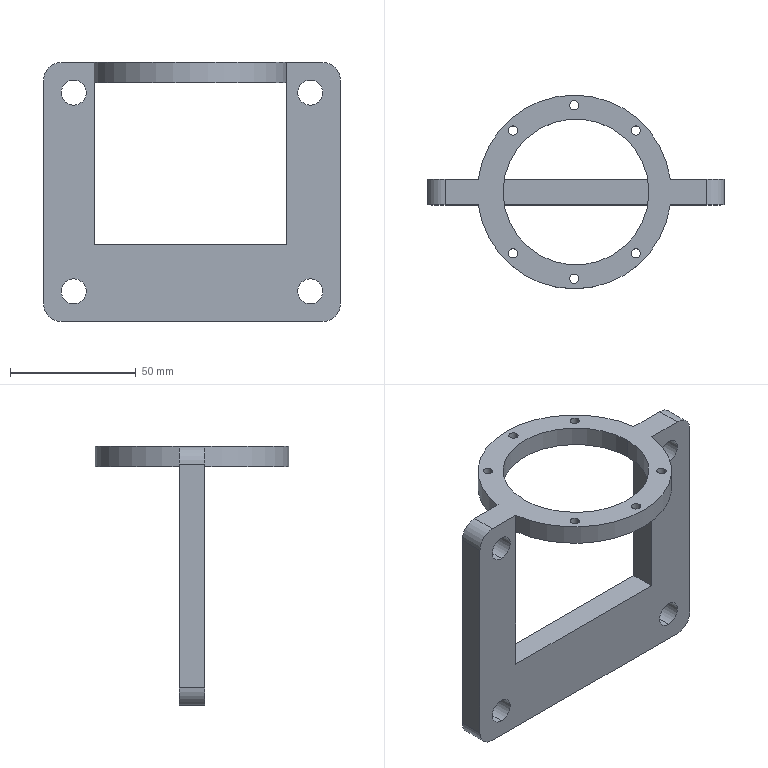Part | SolidWorks | features ICE 4, Extrusion 1, Fillet 1 | 1 solid | 38 faces | box 118 x 77 x 103 mm | volume 78200 mm3 | cylinder 28 | plane 10 | commonest cylinder face diameters 3.7 x12 10 x8 14 x4 58 x2 77 x2
STEP:
#1=CARTESIAN_POINT('',(-46.321,-5.,-9.));
#2=VERTEX_POINT('',#1);
#3=CARTESIAN_POINT('',(-46.321,-5.,1.));
#4=VERTEX_POINT('',#3);
#5=CARTESIAN_POINT('',(-46.321,-5.,-4.));
#6=DIRECTION('',(0.,1.,0.));
#7=DIRECTION('',(0.,0.,-1.));
#8=AXIS2_PLACEMENT_3D('',#5,#6,#7);
#9=CIRCLE('',#8,5.);
#10=EDGE_CURVE('',#2,#4,#9,.T.);
#11=ORIENTED_EDGE('',*,*,#10,.F.);
#12=CARTESIAN_POINT('',(-46.321,5.,-9.));
#13=VERTEX_POINT('',#12);
#14=CARTESIAN_POINT('',(-46.321,-38.501,-9.));
#15=DIRECTION('',(0.,1.,0.));
#16=VECTOR('',#15,1000.);
#17=LINE('',#14,#16);
#18=EDGE_CURVE('',#2,#13,#17,.T.);
#19=ORIENTED_EDGE('',*,*,#18,.T.);
#20=CARTESIAN_POINT('',(-46.321,5.,1.));
#21=VERTEX_POINT('',#20);
#22=CARTESIAN_POINT('',(-46.321,5.,-4.));
#23=DIRECTION('',(0.,1.,0.));
#24=DIRECTION('',(0.,0.,1.));
#25=AXIS2_PLACEMENT_3D('',#22,#23,#24);
#26=CIRCLE('',#25,5.);
#27=EDGE_CURVE('',#13,#21,#26,.T.);
#28=ORIENTED_EDGE('',*,*,#27,.T.);
#29=CARTESIAN_POINT('',(-46.321,-38.501,1.));
#30=DIRECTION('',(0.,1.,0.));
#31=VECTOR('',#30,1000.);
#32=LINE('',#29,#31);
#33=EDGE_CURVE('',#4,#21,#32,.T.);
#34=ORIENTED_EDGE('',*,*,#33,.F.);
#35=EDGE_LOOP('',(#11,#19,#28,#34));
#36=FACE_OUTER_BOUND('',#35,.T.);
#37=CARTESIAN_POINT('',(-46.321,-38.501,-4.));
#38=DIRECTION('',(0.,1.,0.));
#39=DIRECTION('',(0.,0.,1.));
#40=AXIS2_PLACEMENT_3D('',#37,#38,#39);
#41=CYLINDRICAL_SURFACE('',#40,5.);
#42=ADVANCED_FACE('',(#36),#41,.F.);
#43=CARTESIAN_POINT('',(47.679,-5.,-88.));
#44=VERTEX_POINT('',#43);
#45=CARTESIAN_POINT('',(47.679,-5.,-78.));
#46=VERTEX_POINT('',#45);
#47=CARTESIAN_POINT('',(47.679,-5.,-83.));
#48=DIRECTION('',(0.,1.,0.));
#49=DIRECTION('',(0.,0.,-1.));
#50=AXIS2_PLACEMENT_3D('',#47,#48,#49);
#51=CIRCLE('',#50,5.);
#52=EDGE_CURVE('',#44,#46,#51,.T.);
#53=ORIENTED_EDGE('',*,*,#52,.F.);
#54=CARTESIAN_POINT('',(47.679,5.,-88.));
#55=VERTEX_POINT('',#54);
#56=CARTESIAN_POINT('',(47.679,-38.501,-88.));
#57=DIRECTION('',(0.,1.,0.));
#58=VECTOR('',#57,1000.);
#59=LINE('',#56,#58);
#60=EDGE_CURVE('',#44,#55,#59,.T.);
#61=ORIENTED_EDGE('',*,*,#60,.T.);
#62=CARTESIAN_POINT('',(47.679,5.,-78.));
#63=VERTEX_POINT('',#62);
#64=CARTESIAN_POINT('',(47.679,5.,-83.));
#65=DIRECTION('',(0.,1.,0.));
#66=DIRECTION('',(0.,0.,1.));
#67=AXIS2_PLACEMENT_3D('',#64,#65,#66);
#68=CIRCLE('',#67,5.);
#69=EDGE_CURVE('',#55,#63,#68,.T.);
#70=ORIENTED_EDGE('',*,*,#69,.T.);
#71=CARTESIAN_POINT('',(47.679,-38.501,-78.));
#72=DIRECTION('',(0.,1.,0.));
#73=VECTOR('',#72,1000.);
#74=LINE('',#71,#73);
#75=EDGE_CURVE('',#46,#63,#74,.T.);
#76=ORIENTED_EDGE('',*,*,#75,.F.);
#77=EDGE_LOOP('',(#53,#61,#70,#76));
#78=FACE_OUTER_BOUND('',#77,.T.);
#79=CARTESIAN_POINT('',(47.679,-38.501,-83.));
#80=DIRECTION('',(0.,1.,0.));
#81=DIRECTION('',(0.,0.,1.));
#82=AXIS2_PLACEMENT_3D('',#79,#80,#81);
#83=CYLINDRICAL_SURFACE('',#82,5.);
#84=ADVANCED_FACE('',(#78),#83,.F.);
#85=CARTESIAN_POINT('',(47.679,-5.,-9.));
#86=VERTEX_POINT('',#85);
#87=CARTESIAN_POINT('',(47.679,-5.,1.));
#88=VERTEX_POINT('',#87);
#89=CARTESIAN_POINT('',(47.679,-5.,-4.));
#90=DIRECTION('',(0.,1.,0.));
#91=DIRECTION('',(0.,0.,-1.));
#92=AXIS2_PLACEMENT_3D('',#89,#90,#91);
#93=CIRCLE('',#92,5.);
#94=EDGE_CURVE('',#86,#88,#93,.T.);
#95=ORIENTED_EDGE('',*,*,#94,.F.);
#96=CARTESIAN_POINT('',(47.679,5.,-9.));
#97=VERTEX_POINT('',#96);
#98=CARTESIAN_POINT('',(47.679,-38.501,-9.));
#99=DIRECTION('',(0.,1.,0.));
#100=VECTOR('',#99,1000.);
#101=LINE('',#98,#100);
#102=EDGE_CURVE('',#86,#97,#101,.T.);
#103=ORIENTED_EDGE('',*,*,#102,.T.);
#104=CARTESIAN_POINT('',(47.679,5.,1.));
#105=VERTEX_POINT('',#104);
#106=CARTESIAN_POINT('',(47.679,5.,-4.));
#107=DIRECTION('',(0.,1.,0.));
#108=DIRECTION('',(0.,0.,1.));
#109=AXIS2_PLACEMENT_3D('',#106,#107,#108);
#110=CIRCLE('',#109,5.);
#111=EDGE_CURVE('',#97,#105,#110,.T.);
#112=ORIENTED_EDGE('',*,*,#111,.T.);
#113=CARTESIAN_POINT('',(47.679,-38.501,1.));
#114=DIRECTION('',(0.,1.,0.));
#115=VECTOR('',#114,1000.);
#116=LINE('',#113,#115);
#117=EDGE_CURVE('',#88,#105,#116,.T.);
#118=ORIENTED_EDGE('',*,*,#117,.F.);
#119=EDGE_LOOP('',(#95,#103,#112,#118));
#120=FACE_OUTER_BOUND('',#119,.T.);
#121=CARTESIAN_POINT('',(47.679,-38.501,-4.));
#122=DIRECTION('',(0.,1.,0.));
#123=DIRECTION('',(0.,0.,1.));
#124=AXIS2_PLACEMENT_3D('',#121,#122,#123);
#125=CYLINDRICAL_SURFACE('',#124,5.);
#126=ADVANCED_FACE('',(#120),#125,.F.);
#127=CARTESIAN_POINT('',(-46.321,-5.,-88.));
#128=VERTEX_POINT('',#127);
#129=CARTESIAN_POINT('',(-46.321,-5.,-78.));
#130=VERTEX_POINT('',#129);
#131=CARTESIAN_POINT('',(-46.321,-5.,-83.));
#132=DIRECTION('',(0.,1.,0.));
#133=DIRECTION('',(0.,0.,-1.));
#134=AXIS2_PLACEMENT_3D('',#131,#132,#133);
#135=CIRCLE('',#134,5.);
#136=EDGE_CURVE('',#128,#130,#135,.T.);
#137=ORIENTED_EDGE('',*,*,#136,.F.);
#138=CARTESIAN_POINT('',(-46.321,5.,-88.));
#139=VERTEX_POINT('',#138);
#140=CARTESIAN_POINT('',(-46.321,-38.501,-88.));
#141=DIRECTION('',(0.,1.,0.));
#142=VECTOR('',#141,1000.);
#143=LINE('',#140,#142);
#144=EDGE_CURVE('',#128,#139,#143,.T.);
#145=ORIENTED_EDGE('',*,*,#144,.T.);
#146=CARTESIAN_POINT('',(-46.321,5.,-78.));
#147=VERTEX_POINT('',#146);
#148=CARTESIAN_POINT('',(-46.321,5.,-83.));
#149=DIRECTION('',(0.,1.,0.));
#150=DIRECTION('',(0.,0.,1.));
#151=AXIS2_PLACEMENT_3D('',#148,#149,#150);
#152=CIRCLE('',#151,5.);
#153=EDGE_CURVE('',#139,#147,#152,.T.);
#154=ORIENTED_EDGE('',*,*,#153,.T.);
#155=CARTESIAN_POINT('',(-46.321,-38.501,-78.));
#156=DIRECTION('',(0.,1.,0.));
#157=VECTOR('',#156,1000.);
#158=LINE('',#155,#157);
#159=EDGE_CURVE('',#130,#147,#158,.T.);
#160=ORIENTED_EDGE('',*,*,#159,.F.);
#161=EDGE_LOOP('',(#137,#145,#154,#160));
#162=FACE_OUTER_BOUND('',#161,.T.);
#163=CARTESIAN_POINT('',(-46.321,-38.501,-83.));
#164=DIRECTION('',(0.,1.,0.));
#165=DIRECTION('',(0.,0.,1.));
#166=AXIS2_PLACEMENT_3D('',#163,#164,#165);
#167=CYLINDRICAL_SURFACE('',#166,5.);
#168=ADVANCED_FACE('',(#162),#167,.F.);
#169=CARTESIAN_POINT('',(-26.245,24.395,8.));
#170=VERTEX_POINT('',#169);
#171=CARTESIAN_POINT('',(-22.545,24.395,8.));
#172=VERTEX_POINT('',#171);
#173=CARTESIAN_POINT('',(-24.395,24.395,8.));
#174=DIRECTION('',(0.,0.,1.));
#175=DIRECTION('',(1.,0.,0.));
#176=AXIS2_PLACEMENT_3D('',#173,#174,#175);
#177=CIRCLE('',#176,1.85);
#178=EDGE_CURVE('',#170,#172,#177,.T.);
#179=ORIENTED_EDGE('',*,*,#178,.T.);
#180=CARTESIAN_POINT('',(-22.545,24.395,0.));
#181=VERTEX_POINT('',#180);
#182=CARTESIAN_POINT('',(-22.545,24.395,8.));
#183=DIRECTION('',(0.,0.,-1.));
#184=VECTOR('',#183,1000.);
#185=LINE('',#182,#184);
#186=EDGE_CURVE('',#172,#181,#185,.T.);
#187=ORIENTED_EDGE('',*,*,#186,.T.);
#188=CARTESIAN_POINT('',(-26.245,24.395,0.));
#189=VERTEX_POINT('',#188);
#190=CARTESIAN_POINT('',(-24.395,24.395,0.));
#191=DIRECTION('',(0.,0.,1.));
#192=DIRECTION('',(1.,0.,0.));
#193=AXIS2_PLACEMENT_3D('',#190,#191,#192);
#194=CIRCLE('',#193,1.85);
#195=EDGE_CURVE('',#189,#181,#194,.T.);
#196=ORIENTED_EDGE('',*,*,#195,.F.);
#197=CARTESIAN_POINT('',(-26.245,24.395,8.));
#198=DIRECTION('',(0.,0.,-1.));
#199=VECTOR('',#198,1000.);
#200=LINE('',#197,#199);
#201=EDGE_CURVE('',#170,#189,#200,.T.);
#202=ORIENTED_EDGE('',*,*,#201,.F.);
#203=EDGE_LOOP('',(#179,#187,#196,#202));
#204=FACE_OUTER_BOUND('',#203,.T.);
#205=CARTESIAN_POINT('',(-24.395,24.395,8.));
#206=DIRECTION('',(0.,0.,-1.));
#207=DIRECTION('',(-1.,0.,0.));
#208=AXIS2_PLACEMENT_3D('',#205,#206,#207);
#209=CYLINDRICAL_SURFACE('',#208,1.85);
#210=ADVANCED_FACE('',(#204),#209,.F.);
#211=CARTESIAN_POINT('',(-26.245,-24.395,8.));
#212=VERTEX_POINT('',#211);
#213=CARTESIAN_POINT('',(-22.545,-24.395,8.));
#214=VERTEX_POINT('',#213);
#215=CARTESIAN_POINT('',(-24.395,-24.395,8.));
#216=DIRECTION('',(0.,0.,1.));
#217=DIRECTION('',(1.,0.,0.));
#218=AXIS2_PLACEMENT_3D('',#215,#216,#217);
#219=CIRCLE('',#218,1.85);
#220=EDGE_CURVE('',#212,#214,#219,.T.);
#221=ORIENTED_EDGE('',*,*,#220,.T.);
#222=CARTESIAN_POINT('',(-22.545,-24.395,0.));
#223=VERTEX_POINT('',#222);
#224=CARTESIAN_POINT('',(-22.545,-24.395,8.));
#225=DIRECTION('',(0.,0.,-1.));
#226=VECTOR('',#225,1000.);
#227=LINE('',#224,#226);
#228=EDGE_CURVE('',#214,#223,#227,.T.);
#229=ORIENTED_EDGE('',*,*,#228,.T.);
#230=CARTESIAN_POINT('',(-26.245,-24.395,0.));
#231=VERTEX_POINT('',#230);
#232=CARTESIAN_POINT('',(-24.395,-24.395,0.));
#233=DIRECTION('',(0.,0.,1.));
#234=DIRECTION('',(1.,0.,0.));
#235=AXIS2_PLACEMENT_3D('',#232,#233,#234);
#236=CIRCLE('',#235,1.85);
#237=EDGE_CURVE('',#231,#223,#236,.T.);
#238=ORIENTED_EDGE('',*,*,#237,.F.);
#239=CARTESIAN_POINT('',(-26.245,-24.395,8.));
#240=DIRECTION('',(0.,0.,-1.));
#241=VECTOR('',#240,1000.);
#242=LINE('',#239,#241);
#243=EDGE_CURVE('',#212,#231,#242,.T.);
#244=ORIENTED_EDGE('',*,*,#243,.F.);
#245=EDGE_LOOP('',(#221,#229,#238,#244));
#246=FACE_OUTER_BOUND('',#245,.T.);
#247=CARTESIAN_POINT('',(-24.395,-24.395,8.));
#248=DIRECTION('',(0.,0.,-1.));
#249=DIRECTION('',(-1.,0.,0.));
#250=AXIS2_PLACEMENT_3D('',#247,#248,#249);
#251=CYLINDRICAL_SURFACE('',#250,1.85);
#252=ADVANCED_FACE('',(#246),#251,.F.);
#253=CARTESIAN_POINT('',(-1.85,-34.5,8.));
#254=VERTEX_POINT('',#253);
#255=CARTESIAN_POINT('',(1.85,-34.5,8.));
#256=VERTEX_POINT('',#255);
#257=CARTESIAN_POINT('',(0.,-34.5,8.));
#258=DIRECTION('',(0.,0.,1.));
#259=DIRECTION('',(1.,0.,0.));
#260=AXIS2_PLACEMENT_3D('',#257,#258,#259);
#261=CIRCLE('',#260,1.85);
#262=EDGE_CURVE('',#254,#256,#261,.T.);
#263=ORIENTED_EDGE('',*,*,#262,.T.);
#264=CARTESIAN_POINT('',(1.85,-34.5,0.));
#265=VERTEX_POINT('',#264);
#266=CARTESIAN_POINT('',(1.85,-34.5,8.));
#267=DIRECTION('',(0.,0.,-1.));
#268=VECTOR('',#267,1000.);
#269=LINE('',#266,#268);
#270=EDGE_CURVE('',#256,#265,#269,.T.);
#271=ORIENTED_EDGE('',*,*,#270,.T.);
#272=CARTESIAN_POINT('',(-1.85,-34.5,0.));
#273=VERTEX_POINT('',#272);
#274=CARTESIAN_POINT('',(0.,-34.5,0.));
#275=DIRECTION('',(0.,0.,1.));
#276=DIRECTION('',(1.,0.,0.));
#277=AXIS2_PLACEMENT_3D('',#274,#275,#276);
#278=CIRCLE('',#277,1.85);
#279=EDGE_CURVE('',#273,#265,#278,.T.);
#280=ORIENTED_EDGE('',*,*,#279,.F.);
#281=CARTESIAN_POINT('',(-1.85,-34.5,8.));
#282=DIRECTION('',(0.,0.,-1.));
#283=VECTOR('',#282,1000.);
#284=LINE('',#281,#283);
#285=EDGE_CURVE('',#254,#273,#284,.T.);
#286=ORIENTED_EDGE('',*,*,#285,.F.);
#287=EDGE_LOOP('',(#263,#271,#280,#286));
#288=FACE_OUTER_BOUND('',#287,.T.);
#289=CARTESIAN_POINT('',(0.,-34.5,8.));
#290=DIRECTION('',(0.,0.,-1.));
#291=DIRECTION('',(-1.,0.,0.));
#292=AXIS2_PLACEMENT_3D('',#289,#290,#291);
#293=CYLINDRICAL_SURFACE('',#292,1.85);
#294=ADVANCED_FACE('',(#288),#293,.F.);
#295=CARTESIAN_POINT('',(22.545,-24.395,8.));
#296=VERTEX_POINT('',#295);
#297=CARTESIAN_POINT('',(26.245,-24.395,8.));
#298=VERTEX_POINT('',#297);
#299=CARTESIAN_POINT('',(24.395,-24.395,8.));
#300=DIRECTION('',(0.,0.,1.));
#301=DIRECTION('',(1.,0.,0.));
#302=AXIS2_PLACEMENT_3D('',#299,#300,#301);
#303=CIRCLE('',#302,1.85);
#304=EDGE_CURVE('',#296,#298,#303,.T.);
#305=ORIENTED_EDGE('',*,*,#304,.T.);
#306=CARTESIAN_POINT('',(26.245,-24.395,0.));
#307=VERTEX_POINT('',#306);
#308=CARTESIAN_POINT('',(26.245,-24.395,8.));
#309=DIRECTION('',(0.,0.,-1.));
#310=VECTOR('',#309,1000.);
#311=LINE('',#308,#310);
#312=EDGE_CURVE('',#298,#307,#311,.T.);
#313=ORIENTED_EDGE('',*,*,#312,.T.);
#314=CARTESIAN_POINT('',(22.545,-24.395,0.));
#315=VERTEX_POINT('',#314);
#316=CARTESIAN_POINT('',(24.395,-24.395,0.));
#317=DIRECTION('',(0.,0.,1.));
#318=DIRECTION('',(1.,0.,0.));
#319=AXIS2_PLACEMENT_3D('',#316,#317,#318);
#320=CIRCLE('',#319,1.85);
#321=EDGE_CURVE('',#315,#307,#320,.T.);
#322=ORIENTED_EDGE('',*,*,#321,.F.);
#323=CARTESIAN_POINT('',(22.545,-24.395,8.));
#324=DIRECTION('',(0.,0.,-1.));
#325=VECTOR('',#324,1000.);
#326=LINE('',#323,#325);
#327=EDGE_CURVE('',#296,#315,#326,.T.);
#328=ORIENTED_EDGE('',*,*,#327,.F.);
#329=EDGE_LOOP('',(#305,#313,#322,#328));
#330=FACE_OUTER_BOUND('',#329,.T.);
#331=CARTESIAN_POINT('',(24.395,-24.395,8.));
#332=DIRECTION('',(0.,0.,-1.));
#333=DIRECTION('',(-1.,0.,0.));
#334=AXIS2_PLACEMENT_3D('',#331,#332,#333);
#335=CYLINDRICAL_SURFACE('',#334,1.85);
#336=ADVANCED_FACE('',(#330),#335,.F.);
#337=CARTESIAN_POINT('',(22.545,24.395,8.));
#338=VERTEX_POINT('',#337);
#339=CARTESIAN_POINT('',(26.245,24.395,8.));
#340=VERTEX_POINT('',#339);
#341=CARTESIAN_POINT('',(24.395,24.395,8.));
#342=DIRECTION('',(0.,0.,1.));
#343=DIRECTION('',(1.,0.,0.));
#344=AXIS2_PLACEMENT_3D('',#341,#342,#343);
#345=CIRCLE('',#344,1.85);
#346=EDGE_CURVE('',#338,#340,#345,.T.);
#347=ORIENTED_EDGE('',*,*,#346,.T.);
#348=CARTESIAN_POINT('',(26.245,24.395,0.));
#349=VERTEX_POINT('',#348);
#350=CARTESIAN_POINT('',(26.245,24.395,8.));
#351=DIRECTION('',(0.,0.,-1.));
#352=VECTOR('',#351,1000.);
#353=LINE('',#350,#352);
#354=EDGE_CURVE('',#340,#349,#353,.T.);
#355=ORIENTED_EDGE('',*,*,#354,.T.);
#356=CARTESIAN_POINT('',(22.545,24.395,0.));
#357=VERTEX_POINT('',#356);
#358=CARTESIAN_POINT('',(24.395,24.395,0.));
#359=DIRECTION('',(0.,0.,1.));
#360=DIRECTION('',(1.,0.,0.));
#361=AXIS2_PLACEMENT_3D('',#358,#359,#360);
#362=CIRCLE('',#361,1.85);
#363=EDGE_CURVE('',#357,#349,#362,.T.);
#364=ORIENTED_EDGE('',*,*,#363,.F.);
#365=CARTESIAN_POINT('',(22.545,24.395,8.));
#366=DIRECTION('',(0.,0.,-1.));
#367=VECTOR('',#366,1000.);
#368=LINE('',#365,#367);
#369=EDGE_CURVE('',#338,#357,#368,.T.);
#370=ORIENTED_EDGE('',*,*,#369,.F.);
#371=EDGE_LOOP('',(#347,#355,#364,#370));
#372=FACE_OUTER_BOUND('',#371,.T.);
#373=CARTESIAN_POINT('',(24.395,24.395,8.));
#374=DIRECTION('',(0.,0.,-1.));
#375=DIRECTION('',(-1.,0.,0.));
#376=AXIS2_PLACEMENT_3D('',#373,#374,#375);
#377=CYLINDRICAL_SURFACE('',#376,1.85);
#378=ADVANCED_FACE('',(#372),#377,.F.);
#379=CARTESIAN_POINT('',(-1.85,34.5,8.));
#380=VERTEX_POINT('',#379);
#381=CARTESIAN_POINT('',(1.85,34.5,8.));
#382=VERTEX_POINT('',#381);
#383=CARTESIAN_POINT('',(0.,34.5,8.));
#384=DIRECTION('',(0.,0.,1.));
#385=DIRECTION('',(1.,0.,0.));
#386=AXIS2_PLACEMENT_3D('',#383,#384,#385);
#387=CIRCLE('',#386,1.85);
#388=EDGE_CURVE('',#380,#382,#387,.T.);
#389=ORIENTED_EDGE('',*,*,#388,.T.);
#390=CARTESIAN_POINT('',(1.85,34.5,0.));
#391=VERTEX_POINT('',#390);
#392=CARTESIAN_POINT('',(1.85,34.5,8.));
#393=DIRECTION('',(0.,0.,-1.));
#394=VECTOR('',#393,1000.);
#395=LINE('',#392,#394);
#396=EDGE_CURVE('',#382,#391,#395,.T.);
#397=ORIENTED_EDGE('',*,*,#396,.T.);
#398=CARTESIAN_POINT('',(-1.85,34.5,0.));
#399=VERTEX_POINT('',#398);
#400=CARTESIAN_POINT('',(0.,34.5,0.));
#401=DIRECTION('',(0.,0.,1.));
#402=DIRECTION('',(1.,0.,0.));
#403=AXIS2_PLACEMENT_3D('',#400,#401,#402);
#404=CIRCLE('',#403,1.85);
#405=EDGE_CURVE('',#399,#391,#404,.T.);
#406=ORIENTED_EDGE('',*,*,#405,.F.);
#407=CARTESIAN_POINT('',(-1.85,34.5,8.));
#408=DIRECTION('',(0.,0.,-1.));
#409=VECTOR('',#408,1000.);
#410=LINE('',#407,#409);
#411=EDGE_CURVE('',#380,#399,#410,.T.);
#412=ORIENTED_EDGE('',*,*,#411,.F.);
#413=EDGE_LOOP('',(#389,#397,#406,#412));
#414=FACE_OUTER_BOUND('',#413,.T.);
#415=CARTESIAN_POINT('',(0.,34.5,8.));
#416=DIRECTION('',(0.,0.,-1.));
#417=DIRECTION('',(-1.,0.,0.));
#418=AXIS2_PLACEMENT_3D('',#415,#416,#417);
#419=CYLINDRICAL_SURFACE('',#418,1.85);
#420=ADVANCED_FACE('',(#414),#419,.F.);
#421=CARTESIAN_POINT('',(-28.321,0.,8.));
#422=VERTEX_POINT('',#421);
#423=CARTESIAN_POINT('',(29.679,0.,8.));
#424=VERTEX_POINT('',#423);
#425=CARTESIAN_POINT('',(0.6786,0.,8.));
#426=DIRECTION('',(0.,0.,1.));
#427=DIRECTION('',(1.,0.,0.));
#428=AXIS2_PLACEMENT_3D('',#425,#426,#427);
#429=CIRCLE('',#428,29.);
#430=EDGE_CURVE('',#422,#424,#429,.T.);
#431=ORIENTED_EDGE('',*,*,#430,.T.);
#432=CARTESIAN_POINT('',(29.679,0.,0.));
#433=VERTEX_POINT('',#432);
#434=CARTESIAN_POINT('',(29.679,0.,8.));
#435=DIRECTION('',(0.,0.,-1.));
#436=VECTOR('',#435,1000.);
#437=LINE('',#434,#436);
#438=EDGE_CURVE('',#424,#433,#437,.T.);
#439=ORIENTED_EDGE('',*,*,#438,.T.);
#440=CARTESIAN_POINT('',(-28.321,0.,0.));
#441=VERTEX_POINT('',#440);
#442=CARTESIAN_POINT('',(0.6786,0.,0.));
#443=DIRECTION('',(0.,0.,1.));
#444=DIRECTION('',(1.,0.,0.));
#445=AXIS2_PLACEMENT_3D('',#442,#443,#444);
#446=CIRCLE('',#445,29.);
#447=EDGE_CURVE('',#441,#433,#446,.T.);
#448=ORIENTED_EDGE('',*,*,#447,.F.);
#449=CARTESIAN_POINT('',(-28.321,0.,8.));
#450=DIRECTION('',(0.,0.,-1.));
#451=VECTOR('',#450,1000.);
#452=LINE('',#449,#451);
#453=EDGE_CURVE('',#422,#441,#452,.T.);
#454=ORIENTED_EDGE('',*,*,#453,.F.);
#455=EDGE_LOOP('',(#431,#439,#448,#454));
#456=FACE_OUTER_BOUND('',#455,.T.);
#457=CARTESIAN_POINT('',(0.6786,0.,8.));
#458=DIRECTION('',(0.,0.,-1.));
#459=DIRECTION('',(-1.,0.,0.));
#460=AXIS2_PLACEMENT_3D('',#457,#458,#459);
#461=CYLINDRICAL_SURFACE('',#460,29.);
#462=ADVANCED_FACE('',(#456),#461,.F.);
#463=CARTESIAN_POINT('',(-38.174,-5.,0.));
#464=VERTEX_POINT('',#463);
#465=CARTESIAN_POINT('',(-38.174,-5.,8.));
#466=VERTEX_POINT('',#465);
#467=CARTESIAN_POINT('',(-38.174,-5.,8.));
#468=DIRECTION('',(0.,0.,1.));
#469=VECTOR('',#468,1000.);
#470=LINE('',#467,#469);
#471=EDGE_CURVE('',#464,#466,#470,.T.);
#472=ORIENTED_EDGE('',*,*,#471,.F.);
#473=CARTESIAN_POINT('',(38.174,-5.,0.));
#474=VERTEX_POINT('',#473);
#475=CARTESIAN_POINT('',(0.,0.,0.));
#476=DIRECTION('',(0.,0.,1.));
#477=DIRECTION('',(1.,0.,0.));
#478=AXIS2_PLACEMENT_3D('',#475,#476,#477);
#479=CIRCLE('',#478,38.5);
#480=EDGE_CURVE('',#464,#474,#479,.T.);
#481=ORIENTED_EDGE('',*,*,#480,.T.);
#482=CARTESIAN_POINT('',(38.174,-5.,8.));
#483=VERTEX_POINT('',#482);
#484=CARTESIAN_POINT('',(38.174,-5.,8.));
#485=DIRECTION('',(0.,0.,-1.));
#486=VECTOR('',#485,1000.);
#487=LINE('',#484,#486);
#488=EDGE_CURVE('',#483,#474,#487,.T.);
#489=ORIENTED_EDGE('',*,*,#488,.F.);
#490=CARTESIAN_POINT('',(0.,0.,8.));
#491=DIRECTION('',(0.,0.,1.));
#492=DIRECTION('',(1.,0.,0.));
#493=AXIS2_PLACEMENT_3D('',#490,#491,#492);
#494=CIRCLE('',#493,38.5);
#495=EDGE_CURVE('',#466,#483,#494,.T.);
#496=ORIENTED_EDGE('',*,*,#495,.F.);
#497=EDGE_LOOP('',(#472,#481,#489,#496));
#498=FACE_OUTER_BOUND('',#497,.T.);
#499=CARTESIAN_POINT('',(0.,0.,8.));
#500=DIRECTION('',(0.,0.,-1.));
#501=DIRECTION('',(-1.,0.,0.));
#502=AXIS2_PLACEMENT_3D('',#499,#500,#501);
#503=CYLINDRICAL_SURFACE('',#502,38.5);
#504=ADVANCED_FACE('',(#498),#503,.T.);
#505=CARTESIAN_POINT('',(-38.174,5.,8.));
#506=VERTEX_POINT('',#505);
#507=CARTESIAN_POINT('',(-38.174,5.,0.));
#508=VERTEX_POINT('',#507);
#509=CARTESIAN_POINT('',(-38.174,5.,8.));
#510=DIRECTION('',(0.,0.,-1.));
#511=VECTOR('',#510,1000.);
#512=LINE('',#509,#511);
#513=EDGE_CURVE('',#506,#508,#512,.T.);
#514=ORIENTED_EDGE('',*,*,#513,.F.);
#515=CARTESIAN_POINT('',(38.174,5.,8.));
#516=VERTEX_POINT('',#515);
#517=CARTESIAN_POINT('',(0.,0.,8.));
#518=DIRECTION('',(0.,0.,1.));
#519=DIRECTION('',(1.,0.,0.));
#520=AXIS2_PLACEMENT_3D('',#517,#518,#519);
#521=CIRCLE('',#520,38.5);
#522=EDGE_CURVE('',#516,#506,#521,.T.);
#523=ORIENTED_EDGE('',*,*,#522,.F.);
#524=CARTESIAN_POINT('',(38.174,5.,0.));
#525=VERTEX_POINT('',#524);
#526=CARTESIAN_POINT('',(38.174,5.,8.));
#527=DIRECTION('',(0.,0.,1.));
#528=VECTOR('',#527,1000.);
#529=LINE('',#526,#528);
#530=EDGE_CURVE('',#525,#516,#529,.T.);
#531=ORIENTED_EDGE('',*,*,#530,.F.);
#532=CARTESIAN_POINT('',(0.,0.,0.));
#533=DIRECTION('',(0.,0.,1.));
#534=DIRECTION('',(1.,0.,0.));
#535=AXIS2_PLACEMENT_3D('',#532,#533,#534);
#536=CIRCLE('',#535,38.5);
#537=EDGE_CURVE('',#525,#508,#536,.T.);
#538=ORIENTED_EDGE('',*,*,#537,.T.);
#539=EDGE_LOOP('',(#514,#523,#531,#538));
#540=FACE_OUTER_BOUND('',#539,.T.);
#541=CARTESIAN_POINT('',(0.,0.,8.));
#542=DIRECTION('',(0.,0.,-1.));
#543=DIRECTION('',(-1.,0.,0.));
#544=AXIS2_PLACEMENT_3D('',#541,#542,#543);
#545=CYLINDRICAL_SURFACE('',#544,38.5);
#546=ADVANCED_FACE('',(#540),#545,.T.);
#547=CARTESIAN_POINT('',(52.679,-5.,8.));
#548=VERTEX_POINT('',#547);
#549=CARTESIAN_POINT('',(33.981,-5.,8.));
#550=DIRECTION('',(1.,0.,0.));
#551=VECTOR('',#550,1000.);
#552=LINE('',#549,#551);
#553=EDGE_CURVE('',#483,#548,#552,.T.);
#554=ORIENTED_EDGE('',*,*,#553,.T.);
#555=CARTESIAN_POINT('',(52.679,5.,8.));
#556=VERTEX_POINT('',#555);
#557=CARTESIAN_POINT('',(52.679,0.,8.));
#558=DIRECTION('',(0.,1.,0.));
#559=VECTOR('',#558,1000.);
#560=LINE('',#557,#559);
#561=EDGE_CURVE('',#548,#556,#560,.T.);
#562=ORIENTED_EDGE('',*,*,#561,.T.);
#563=CARTESIAN_POINT('',(59.679,5.,8.));
#564=DIRECTION('',(-1.,0.,0.));
#565=VECTOR('',#564,1000.);
#566=LINE('',#563,#565);
#567=EDGE_CURVE('',#556,#516,#566,.T.);
#568=ORIENTED_EDGE('',*,*,#567,.T.);
#569=ORIENTED_EDGE('',*,*,#522,.T.);
#570=CARTESIAN_POINT('',(-51.321,5.,8.));
#571=VERTEX_POINT('',#570);
#572=CARTESIAN_POINT('',(-58.321,5.,8.));
#573=DIRECTION('',(-1.,0.,0.));
#574=VECTOR('',#573,1000.);
#575=LINE('',#572,#574);
#576=EDGE_CURVE('',#506,#571,#575,.T.);
#577=ORIENTED_EDGE('',*,*,#576,.T.);
#578=CARTESIAN_POINT('',(-51.321,-5.,8.));
#579=VERTEX_POINT('',#578);
#580=CARTESIAN_POINT('',(-51.321,0.,8.));
#581=DIRECTION('',(0.,-1.,0.));
#582=VECTOR('',#581,1000.);
#583=LINE('',#580,#582);
#584=EDGE_CURVE('',#571,#579,#583,.T.);
#585=ORIENTED_EDGE('',*,*,#584,.T.);
#586=CARTESIAN_POINT('',(-35.407,-5.,8.));
#587=DIRECTION('',(1.,0.,0.));
#588=VECTOR('',#587,1000.);
#589=LINE('',#586,#588);
#590=EDGE_CURVE('',#579,#466,#589,.T.);
#591=ORIENTED_EDGE('',*,*,#590,.T.);
#592=ORIENTED_EDGE('',*,*,#495,.T.);
#593=EDGE_LOOP('',(#554,#562,#568,#569,#577,#585,#591,#592));
#594=FACE_OUTER_BOUND('',#593,.T.);
#595=ORIENTED_EDGE('',*,*,#220,.F.);
#596=CARTESIAN_POINT('',(-24.395,-24.395,8.));
#597=DIRECTION('',(0.,0.,1.));
#598=DIRECTION('',(1.,0.,0.));
#599=AXIS2_PLACEMENT_3D('',#596,#597,#598);
#600=CIRCLE('',#599,1.85);
#601=EDGE_CURVE('',#214,#212,#600,.T.);
#602=ORIENTED_EDGE('',*,*,#601,.F.);
#603=EDGE_LOOP('',(#595,#602));
#604=FACE_BOUND('',#603,.T.);
#605=ORIENTED_EDGE('',*,*,#304,.F.);
#606=CARTESIAN_POINT('',(24.395,-24.395,8.));
#607=DIRECTION('',(0.,0.,1.));
#608=DIRECTION('',(1.,0.,0.));
#609=AXIS2_PLACEMENT_3D('',#606,#607,#608);
#610=CIRCLE('',#609,1.85);
#611=EDGE_CURVE('',#298,#296,#610,.T.);
#612=ORIENTED_EDGE('',*,*,#611,.F.);
#613=EDGE_LOOP('',(#605,#612));
#614=FACE_BOUND('',#613,.T.);
#615=ORIENTED_EDGE('',*,*,#388,.F.);
#616=CARTESIAN_POINT('',(0.,34.5,8.));
#617=DIRECTION('',(0.,0.,1.));
#618=DIRECTION('',(1.,0.,0.));
#619=AXIS2_PLACEMENT_3D('',#616,#617,#618);
#620=CIRCLE('',#619,1.85);
#621=EDGE_CURVE('',#382,#380,#620,.T.);
#622=ORIENTED_EDGE('',*,*,#621,.F.);
#623=EDGE_LOOP('',(#615,#622));
#624=FACE_BOUND('',#623,.T.);
#625=ORIENTED_EDGE('',*,*,#430,.F.);
#626=CARTESIAN_POINT('',(0.6786,0.,8.));
#627=DIRECTION('',(0.,0.,1.));
#628=DIRECTION('',(1.,0.,0.));
#629=AXIS2_PLACEMENT_3D('',#626,#627,#628);
#630=CIRCLE('',#629,29.);
#631=EDGE_CURVE('',#424,#422,#630,.T.);
#632=ORIENTED_EDGE('',*,*,#631,.F.);
#633=EDGE_LOOP('',(#625,#632));
#634=FACE_BOUND('',#633,.T.);
#635=ORIENTED_EDGE('',*,*,#346,.F.);
#636=CARTESIAN_POINT('',(24.395,24.395,8.));
#637=DIRECTION('',(0.,0.,1.));
#638=DIRECTION('',(1.,0.,0.));
#639=AXIS2_PLACEMENT_3D('',#636,#637,#638);
#640=CIRCLE('',#639,1.85);
#641=EDGE_CURVE('',#340,#338,#640,.T.);
#642=ORIENTED_EDGE('',*,*,#641,.F.);
#643=EDGE_LOOP('',(#635,#642));
#644=FACE_BOUND('',#643,.T.);
#645=ORIENTED_EDGE('',*,*,#262,.F.);
#646=CARTESIAN_POINT('',(0.,-34.5,8.));
#647=DIRECTION('',(0.,0.,1.));
#648=DIRECTION('',(1.,0.,0.));
#649=AXIS2_PLACEMENT_3D('',#646,#647,#648);
#650=CIRCLE('',#649,1.85);
#651=EDGE_CURVE('',#256,#254,#650,.T.);
#652=ORIENTED_EDGE('',*,*,#651,.F.);
#653=EDGE_LOOP('',(#645,#652));
#654=FACE_BOUND('',#653,.T.);
#655=ORIENTED_EDGE('',*,*,#178,.F.);
#656=CARTESIAN_POINT('',(-24.395,24.395,8.));
#657=DIRECTION('',(0.,0.,1.));
#658=DIRECTION('',(1.,0.,0.));
#659=AXIS2_PLACEMENT_3D('',#656,#657,#658);
#660=CIRCLE('',#659,1.85);
#661=EDGE_CURVE('',#172,#170,#660,.T.);
#662=ORIENTED_EDGE('',*,*,#661,.F.);
#663=EDGE_LOOP('',(#655,#662));
#664=FACE_BOUND('',#663,.T.);
#665=CARTESIAN_POINT('',(0.,0.,8.));
#666=DIRECTION('',(0.,0.,1.));
#667=DIRECTION('',(1.,0.,0.));
#668=AXIS2_PLACEMENT_3D('',#665,#666,#667);
#669=PLANE('',#668);
#670=ADVANCED_FACE('',(#594,#604,#614,#624,#634,#644,#654,#664),#669,.T.);
#671=ORIENTED_EDGE('',*,*,#447,.T.);
#672=CARTESIAN_POINT('',(0.6786,0.,0.));
#673=DIRECTION('',(0.,0.,1.));
#674=DIRECTION('',(1.,0.,0.));
#675=AXIS2_PLACEMENT_3D('',#672,#673,#674);
#676=CIRCLE('',#675,29.);
#677=EDGE_CURVE('',#433,#441,#676,.T.);
#678=ORIENTED_EDGE('',*,*,#677,.T.);
#679=EDGE_LOOP('',(#671,#678));
#680=FACE_BOUND('',#679,.T.);
#681=ORIENTED_EDGE('',*,*,#480,.F.);
#682=CARTESIAN_POINT('',(-38.174,-38.501,0.));
#683=DIRECTION('',(0.,1.,0.));
#684=VECTOR('',#683,1000.);
#685=LINE('',#682,#684);
#686=EDGE_CURVE('',#464,#508,#685,.T.);
#687=ORIENTED_EDGE('',*,*,#686,.T.);
#688=ORIENTED_EDGE('',*,*,#537,.F.);
#689=CARTESIAN_POINT('',(38.174,-38.501,0.));
#690=DIRECTION('',(0.,1.,0.));
#691=VECTOR('',#690,1000.);
#692=LINE('',#689,#691);
#693=EDGE_CURVE('',#474,#525,#692,.T.);
#694=ORIENTED_EDGE('',*,*,#693,.F.);
#695=EDGE_LOOP('',(#681,#687,#688,#694));
#696=FACE_OUTER_BOUND('',#695,.T.);
#697=ORIENTED_EDGE('',*,*,#405,.T.);
#698=CARTESIAN_POINT('',(0.,34.5,0.));
#699=DIRECTION('',(0.,0.,1.));
#700=DIRECTION('',(1.,0.,0.));
#701=AXIS2_PLACEMENT_3D('',#698,#699,#700);
#702=CIRCLE('',#701,1.85);
#703=EDGE_CURVE('',#391,#399,#702,.T.);
#704=ORIENTED_EDGE('',*,*,#703,.T.);
#705=EDGE_LOOP('',(#697,#704));
#706=FACE_BOUND('',#705,.T.);
#707=ORIENTED_EDGE('',*,*,#363,.T.);
#708=CARTESIAN_POINT('',(24.395,24.395,0.));
#709=DIRECTION('',(0.,0.,1.));
#710=DIRECTION('',(1.,0.,0.));
#711=AXIS2_PLACEMENT_3D('',#708,#709,#710);
#712=CIRCLE('',#711,1.85);
#713=EDGE_CURVE('',#349,#357,#712,.T.);
#714=ORIENTED_EDGE('',*,*,#713,.T.);
#715=EDGE_LOOP('',(#707,#714));
#716=FACE_BOUND('',#715,.T.);
#717=ORIENTED_EDGE('',*,*,#195,.T.);
#718=CARTESIAN_POINT('',(-24.395,24.395,0.));
#719=DIRECTION('',(0.,0.,1.));
#720=DIRECTION('',(1.,0.,0.));
#721=AXIS2_PLACEMENT_3D('',#718,#719,#720);
#722=CIRCLE('',#721,1.85);
#723=EDGE_CURVE('',#181,#189,#722,.T.);
#724=ORIENTED_EDGE('',*,*,#723,.T.);
#725=EDGE_LOOP('',(#717,#724));
#726=FACE_BOUND('',#725,.T.);
#727=ORIENTED_EDGE('',*,*,#237,.T.);
#728=CARTESIAN_POINT('',(-24.395,-24.395,0.));
#729=DIRECTION('',(0.,0.,1.));
#730=DIRECTION('',(1.,0.,0.));
#731=AXIS2_PLACEMENT_3D('',#728,#729,#730);
#732=CIRCLE('',#731,1.85);
#733=EDGE_CURVE('',#223,#231,#732,.T.);
#734=ORIENTED_EDGE('',*,*,#733,.T.);
#735=EDGE_LOOP('',(#727,#734));
#736=FACE_BOUND('',#735,.T.);
#737=ORIENTED_EDGE('',*,*,#279,.T.);
#738=CARTESIAN_POINT('',(0.,-34.5,0.));
#739=DIRECTION('',(0.,0.,1.));
#740=DIRECTION('',(1.,0.,0.));
#741=AXIS2_PLACEMENT_3D('',#738,#739,#740);
#742=CIRCLE('',#741,1.85);
#743=EDGE_CURVE('',#265,#273,#742,.T.);
#744=ORIENTED_EDGE('',*,*,#743,.T.);
#745=EDGE_LOOP('',(#737,#744));
#746=FACE_BOUND('',#745,.T.);
#747=ORIENTED_EDGE('',*,*,#321,.T.);
#748=CARTESIAN_POINT('',(24.395,-24.395,0.));
#749=DIRECTION('',(0.,0.,1.));
#750=DIRECTION('',(1.,0.,0.));
#751=AXIS2_PLACEMENT_3D('',#748,#749,#750);
#752=CIRCLE('',#751,1.85);
#753=EDGE_CURVE('',#307,#315,#752,.T.);
#754=ORIENTED_EDGE('',*,*,#753,.T.);
#755=EDGE_LOOP('',(#747,#754));
#756=FACE_BOUND('',#755,.T.);
#757=CARTESIAN_POINT('',(0.,0.,0.));
#758=DIRECTION('',(0.,0.,1.));
#759=DIRECTION('',(1.,0.,0.));
#760=AXIS2_PLACEMENT_3D('',#757,#758,#759);
#761=PLANE('',#760);
#762=ADVANCED_FACE('',(#680,#696,#706,#716,#726,#736,#746,#756),#761,.F.);
#763=ORIENTED_EDGE('',*,*,#438,.F.);
#764=ORIENTED_EDGE('',*,*,#631,.T.);
#765=ORIENTED_EDGE('',*,*,#453,.T.);
#766=ORIENTED_EDGE('',*,*,#677,.F.);
#767=EDGE_LOOP('',(#763,#764,#765,#766));
#768=FACE_OUTER_BOUND('',#767,.T.);
#769=CARTESIAN_POINT('',(0.6786,0.,8.));
#770=DIRECTION('',(0.,0.,-1.));
#771=DIRECTION('',(-1.,0.,0.));
#772=AXIS2_PLACEMENT_3D('',#769,#770,#771);
#773=CYLINDRICAL_SURFACE('',#772,29.);
#774=ADVANCED_FACE('',(#768),#773,.F.);
#775=ORIENTED_EDGE('',*,*,#396,.F.);
#776=ORIENTED_EDGE('',*,*,#621,.T.);
#777=ORIENTED_EDGE('',*,*,#411,.T.);
#778=ORIENTED_EDGE('',*,*,#703,.F.);
#779=EDGE_LOOP('',(#775,#776,#777,#778));
#780=FACE_OUTER_BOUND('',#779,.T.);
#781=CARTESIAN_POINT('',(0.,34.5,8.));
#782=DIRECTION('',(0.,0.,-1.));
#783=DIRECTION('',(-1.,0.,0.));
#784=AXIS2_PLACEMENT_3D('',#781,#782,#783);
#785=CYLINDRICAL_SURFACE('',#784,1.85);
#786=ADVANCED_FACE('',(#780),#785,.F.);
#787=ORIENTED_EDGE('',*,*,#354,.F.);
#788=ORIENTED_EDGE('',*,*,#641,.T.);
#789=ORIENTED_EDGE('',*,*,#369,.T.);
#790=ORIENTED_EDGE('',*,*,#713,.F.);
#791=EDGE_LOOP('',(#787,#788,#789,#790));
#792=FACE_OUTER_BOUND('',#791,.T.);
#793=CARTESIAN_POINT('',(24.395,24.395,8.));
#794=DIRECTION('',(0.,0.,-1.));
#795=DIRECTION('',(-1.,0.,0.));
#796=AXIS2_PLACEMENT_3D('',#793,#794,#795);
#797=CYLINDRICAL_SURFACE('',#796,1.85);
#798=ADVANCED_FACE('',(#792),#797,.F.);
#799=ORIENTED_EDGE('',*,*,#312,.F.);
#800=ORIENTED_EDGE('',*,*,#611,.T.);
#801=ORIENTED_EDGE('',*,*,#327,.T.);
#802=ORIENTED_EDGE('',*,*,#753,.F.);
#803=EDGE_LOOP('',(#799,#800,#801,#802));
#804=FACE_OUTER_BOUND('',#803,.T.);
#805=CARTESIAN_POINT('',(24.395,-24.395,8.));
#806=DIRECTION('',(0.,0.,-1.));
#807=DIRECTION('',(-1.,0.,0.));
#808=AXIS2_PLACEMENT_3D('',#805,#806,#807);
#809=CYLINDRICAL_SURFACE('',#808,1.85);
#810=ADVANCED_FACE('',(#804),#809,.F.);
#811=ORIENTED_EDGE('',*,*,#270,.F.);
#812=ORIENTED_EDGE('',*,*,#651,.T.);
#813=ORIENTED_EDGE('',*,*,#285,.T.);
#814=ORIENTED_EDGE('',*,*,#743,.F.);
#815=EDGE_LOOP('',(#811,#812,#813,#814));
#816=FACE_OUTER_BOUND('',#815,.T.);
#817=CARTESIAN_POINT('',(0.,-34.5,8.));
#818=DIRECTION('',(0.,0.,-1.));
#819=DIRECTION('',(-1.,0.,0.));
#820=AXIS2_PLACEMENT_3D('',#817,#818,#819);
#821=CYLINDRICAL_SURFACE('',#820,1.85);
#822=ADVANCED_FACE('',(#816),#821,.F.);
#823=ORIENTED_EDGE('',*,*,#228,.F.);
#824=ORIENTED_EDGE('',*,*,#601,.T.);
#825=ORIENTED_EDGE('',*,*,#243,.T.);
#826=ORIENTED_EDGE('',*,*,#733,.F.);
#827=EDGE_LOOP('',(#823,#824,#825,#826));
#828=FACE_OUTER_BOUND('',#827,.T.);
#829=CARTESIAN_POINT('',(-24.395,-24.395,8.));
#830=DIRECTION('',(0.,0.,-1.));
#831=DIRECTION('',(-1.,0.,0.));
#832=AXIS2_PLACEMENT_3D('',#829,#830,#831);
#833=CYLINDRICAL_SURFACE('',#832,1.85);
#834=ADVANCED_FACE('',(#828),#833,.F.);
#835=ORIENTED_EDGE('',*,*,#186,.F.);
#836=ORIENTED_EDGE('',*,*,#661,.T.);
#837=ORIENTED_EDGE('',*,*,#201,.T.);
#838=ORIENTED_EDGE('',*,*,#723,.F.);
#839=EDGE_LOOP('',(#835,#836,#837,#838));
#840=FACE_OUTER_BOUND('',#839,.T.);
#841=CARTESIAN_POINT('',(-24.395,24.395,8.));
#842=DIRECTION('',(0.,0.,-1.));
#843=DIRECTION('',(-1.,0.,0.));
#844=AXIS2_PLACEMENT_3D('',#841,#842,#843);
#845=CYLINDRICAL_SURFACE('',#844,1.85);
#846=ADVANCED_FACE('',(#840),#845,.F.);
#847=CARTESIAN_POINT('',(-58.321,-5.,-88.));
#848=VERTEX_POINT('',#847);
#849=CARTESIAN_POINT('',(-58.321,-5.,1.));
#850=VERTEX_POINT('',#849);
#851=CARTESIAN_POINT('',(-58.321,-5.,-67.773));
#852=DIRECTION('',(0.,0.,1.));
#853=VECTOR('',#852,1000.);
#854=LINE('',#851,#853);
#855=EDGE_CURVE('',#848,#850,#854,.T.);
#856=ORIENTED_EDGE('',*,*,#855,.T.);
#857=CARTESIAN_POINT('',(-58.321,5.,1.));
#858=VERTEX_POINT('',#857);
#859=CARTESIAN_POINT('',(-58.321,-5.,1.));
#860=DIRECTION('',(0.,1.,0.));
#861=VECTOR('',#860,1000.);
#862=LINE('',#859,#861);
#863=EDGE_CURVE('',#850,#858,#862,.T.);
#864=ORIENTED_EDGE('',*,*,#863,.T.);
#865=CARTESIAN_POINT('',(-58.321,5.,-88.));
#866=VERTEX_POINT('',#865);
#867=CARTESIAN_POINT('',(-58.321,5.,-67.773));
#868=DIRECTION('',(0.,0.,1.));
#869=VECTOR('',#868,1000.);
#870=LINE('',#867,#869);
#871=EDGE_CURVE('',#866,#858,#870,.T.);
#872=ORIENTED_EDGE('',*,*,#871,.F.);
#873=CARTESIAN_POINT('',(-58.321,-5.,-88.));
#874=DIRECTION('',(0.,-1.,0.));
#875=VECTOR('',#874,1000.);
#876=LINE('',#873,#875);
#877=EDGE_CURVE('',#866,#848,#876,.T.);
#878=ORIENTED_EDGE('',*,*,#877,.T.);
#879=EDGE_LOOP('',(#856,#864,#872,#878));
#880=FACE_OUTER_BOUND('',#879,.T.);
#881=CARTESIAN_POINT('',(-58.321,-5.,0.));
#882=DIRECTION('',(-1.,0.,0.));
#883=DIRECTION('',(0.,0.,1.));
#884=AXIS2_PLACEMENT_3D('',#881,#882,#883);
#885=PLANE('',#884);
#886=ADVANCED_FACE('',(#880),#885,.T.);
#887=CARTESIAN_POINT('',(52.679,5.,-95.));
#888=VERTEX_POINT('',#887);
#889=CARTESIAN_POINT('',(-51.321,5.,-95.));
#890=VERTEX_POINT('',#889);
#891=CARTESIAN_POINT('',(-58.321,5.,-95.));
#892=DIRECTION('',(-1.,0.,0.));
#893=VECTOR('',#892,1000.);
#894=LINE('',#891,#893);
#895=EDGE_CURVE('',#888,#890,#894,.T.);
#896=ORIENTED_EDGE('',*,*,#895,.F.);
#897=CARTESIAN_POINT('',(52.679,-5.,-95.));
#898=VERTEX_POINT('',#897);
#899=CARTESIAN_POINT('',(52.679,-5.,-95.));
#900=DIRECTION('',(0.,-1.,0.));
#901=VECTOR('',#900,1000.);
#902=LINE('',#899,#901);
#903=EDGE_CURVE('',#888,#898,#902,.T.);
#904=ORIENTED_EDGE('',*,*,#903,.T.);
#905=CARTESIAN_POINT('',(-51.321,-5.,-95.));
#906=VERTEX_POINT('',#905);
#907=CARTESIAN_POINT('',(-58.321,-5.,-95.));
#908=DIRECTION('',(-1.,0.,0.));
#909=VECTOR('',#908,1000.);
#910=LINE('',#907,#909);
#911=EDGE_CURVE('',#898,#906,#910,.T.);
#912=ORIENTED_EDGE('',*,*,#911,.T.);
#913=CARTESIAN_POINT('',(-51.321,-5.,-95.));
#914=DIRECTION('',(0.,1.,0.));
#915=VECTOR('',#914,1000.);
#916=LINE('',#913,#915);
#917=EDGE_CURVE('',#906,#890,#916,.T.);
#918=ORIENTED_EDGE('',*,*,#917,.T.);
#919=EDGE_LOOP('',(#896,#904,#912,#918));
#920=FACE_OUTER_BOUND('',#919,.T.);
#921=CARTESIAN_POINT('',(-58.321,-5.,-95.));
#922=DIRECTION('',(0.,0.,-1.));
#923=DIRECTION('',(-1.,0.,0.));
#924=AXIS2_PLACEMENT_3D('',#921,#922,#923);
#925=PLANE('',#924);
#926=ADVANCED_FACE('',(#920),#925,.T.);
#927=CARTESIAN_POINT('',(59.679,5.,1.));
#928=VERTEX_POINT('',#927);
#929=CARTESIAN_POINT('',(59.679,5.,-88.));
#930=VERTEX_POINT('',#929);
#931=CARTESIAN_POINT('',(59.679,5.,-67.773));
#932=DIRECTION('',(0.,0.,-1.));
#933=VECTOR('',#932,1000.);
#934=LINE('',#931,#933);
#935=EDGE_CURVE('',#928,#930,#934,.T.);
#936=ORIENTED_EDGE('',*,*,#935,.F.);
#937=CARTESIAN_POINT('',(59.679,-5.,1.));
#938=VERTEX_POINT('',#937);
#939=CARTESIAN_POINT('',(59.679,-5.,1.));
#940=DIRECTION('',(0.,-1.,0.));
#941=VECTOR('',#940,1000.);
#942=LINE('',#939,#941);
#943=EDGE_CURVE('',#928,#938,#942,.T.);
#944=ORIENTED_EDGE('',*,*,#943,.T.);
#945=CARTESIAN_POINT('',(59.679,-5.,-88.));
#946=VERTEX_POINT('',#945);
#947=CARTESIAN_POINT('',(59.679,-5.,-67.773));
#948=DIRECTION('',(0.,0.,-1.));
#949=VECTOR('',#948,1000.);
#950=LINE('',#947,#949);
#951=EDGE_CURVE('',#938,#946,#950,.T.);
#952=ORIENTED_EDGE('',*,*,#951,.T.);
#953=CARTESIAN_POINT('',(59.679,-5.,-88.));
#954=DIRECTION('',(0.,1.,0.));
#955=VECTOR('',#954,1000.);
#956=LINE('',#953,#955);
#957=EDGE_CURVE('',#946,#930,#956,.T.);
#958=ORIENTED_EDGE('',*,*,#957,.T.);
#959=EDGE_LOOP('',(#936,#944,#952,#958));
#960=FACE_OUTER_BOUND('',#959,.T.);
#961=CARTESIAN_POINT('',(59.679,-5.,-95.));
#962=DIRECTION('',(1.,0.,0.));
#963=DIRECTION('',(0.,0.,-1.));
#964=AXIS2_PLACEMENT_3D('',#961,#962,#963);
#965=PLANE('',#964);
#966=ADVANCED_FACE('',(#960),#965,.T.);
#967=CARTESIAN_POINT('',(-38.174,-5.,-64.489));
#968=VERTEX_POINT('',#967);
#969=CARTESIAN_POINT('',(-38.174,-5.,0.));
#970=DIRECTION('',(0.,0.,1.));
#971=VECTOR('',#970,1000.);
#972=LINE('',#969,#971);
#973=EDGE_CURVE('',#968,#464,#972,.T.);
#974=ORIENTED_EDGE('',*,*,#973,.T.);
#975=ORIENTED_EDGE('',*,*,#471,.T.);
#976=ORIENTED_EDGE('',*,*,#590,.F.);
#977=CARTESIAN_POINT('',(-51.321,-5.,1.));
#978=DIRECTION('',(0.,-1.,0.));
#979=DIRECTION('',(0.,0.,-1.));
#980=AXIS2_PLACEMENT_3D('',#977,#978,#979);
#981=CIRCLE('',#980,7.);
#982=EDGE_CURVE('',#579,#850,#981,.T.);
#983=ORIENTED_EDGE('',*,*,#982,.T.);
#984=ORIENTED_EDGE('',*,*,#855,.F.);
#985=CARTESIAN_POINT('',(-51.321,-5.,-88.));
#986=DIRECTION('',(0.,-1.,0.));
#987=DIRECTION('',(0.,0.,-1.));
#988=AXIS2_PLACEMENT_3D('',#985,#986,#987);
#989=CIRCLE('',#988,7.);
#990=EDGE_CURVE('',#848,#906,#989,.T.);
#991=ORIENTED_EDGE('',*,*,#990,.T.);
#992=ORIENTED_EDGE('',*,*,#911,.F.);
#993=CARTESIAN_POINT('',(52.679,-5.,-88.));
#994=DIRECTION('',(0.,-1.,0.));
#995=DIRECTION('',(0.,0.,-1.));
#996=AXIS2_PLACEMENT_3D('',#993,#994,#995);
#997=CIRCLE('',#996,7.);
#998=EDGE_CURVE('',#898,#946,#997,.T.);
#999=ORIENTED_EDGE('',*,*,#998,.T.);
#1000=ORIENTED_EDGE('',*,*,#951,.F.);
#1001=CARTESIAN_POINT('',(52.679,-5.,1.));
#1002=DIRECTION('',(0.,-1.,0.));
#1003=DIRECTION('',(0.,0.,-1.));
#1004=AXIS2_PLACEMENT_3D('',#1001,#1002,#1003);
#1005=CIRCLE('',#1004,7.);
#1006=EDGE_CURVE('',#938,#548,#1005,.T.);
#1007=ORIENTED_EDGE('',*,*,#1006,.T.);
#1008=ORIENTED_EDGE('',*,*,#553,.F.);
#1009=ORIENTED_EDGE('',*,*,#488,.T.);
#1010=CARTESIAN_POINT('',(38.174,-5.,-64.489));
#1011=VERTEX_POINT('',#1010);
#1012=CARTESIAN_POINT('',(38.174,-5.,-64.489));
#1013=DIRECTION('',(0.,0.,-1.));
#1014=VECTOR('',#1013,1000.);
#1015=LINE('',#1012,#1014);
#1016=EDGE_CURVE('',#474,#1011,#1015,.T.);
#1017=ORIENTED_EDGE('',*,*,#1016,.T.);
#1018=CARTESIAN_POINT('',(-38.174,-5.,-64.489));
#1019=DIRECTION('',(-1.,0.,0.));
#1020=VECTOR('',#1019,1000.);
#1021=LINE('',#1018,#1020);
#1022=EDGE_CURVE('',#1011,#968,#1021,.T.);
#1023=ORIENTED_EDGE('',*,*,#1022,.T.);
#1024=EDGE_LOOP('',(#974,#975,#976,#983,#984,#991,#992,#999,#1000,#1007,#1008,#1009,#1017,#1023));
#1025=FACE_OUTER_BOUND('',#1024,.T.);
#1026=CARTESIAN_POINT('',(-46.321,-5.,-4.));
#1027=DIRECTION('',(0.,1.,0.));
#1028=DIRECTION('',(0.,0.,-1.));
#1029=AXIS2_PLACEMENT_3D('',#1026,#1027,#1028);
#1030=CIRCLE('',#1029,5.);
#1031=EDGE_CURVE('',#4,#2,#1030,.T.);
#1032=ORIENTED_EDGE('',*,*,#1031,.T.);
#1033=ORIENTED_EDGE('',*,*,#10,.T.);
#1034=EDGE_LOOP('',(#1032,#1033));
#1035=FACE_BOUND('',#1034,.T.);
#1036=CARTESIAN_POINT('',(47.679,-5.,-83.));
#1037=DIRECTION('',(0.,1.,0.));
#1038=DIRECTION('',(0.,0.,-1.));
#1039=AXIS2_PLACEMENT_3D('',#1036,#1037,#1038);
#1040=CIRCLE('',#1039,5.);
#1041=EDGE_CURVE('',#46,#44,#1040,.T.);
#1042=ORIENTED_EDGE('',*,*,#1041,.T.);
#1043=ORIENTED_EDGE('',*,*,#52,.T.);
#1044=EDGE_LOOP('',(#1042,#1043));
#1045=FACE_BOUND('',#1044,.T.);
#1046=CARTESIAN_POINT('',(47.679,-5.,-4.));
#1047=DIRECTION('',(0.,1.,0.));
#1048=DIRECTION('',(0.,0.,-1.));
#1049=AXIS2_PLACEMENT_3D('',#1046,#1047,#1048);
#1050=CIRCLE('',#1049,5.);
#1051=EDGE_CURVE('',#88,#86,#1050,.T.);
#1052=ORIENTED_EDGE('',*,*,#1051,.T.);
#1053=ORIENTED_EDGE('',*,*,#94,.T.);
#1054=EDGE_LOOP('',(#1052,#1053));
#1055=FACE_BOUND('',#1054,.T.);
#1056=CARTESIAN_POINT('',(-46.321,-5.,-83.));
#1057=DIRECTION('',(0.,1.,0.));
#1058=DIRECTION('',(0.,0.,-1.));
#1059=AXIS2_PLACEMENT_3D('',#1056,#1057,#1058);
#1060=CIRCLE('',#1059,5.);
#1061=EDGE_CURVE('',#130,#128,#1060,.T.);
#1062=ORIENTED_EDGE('',*,*,#1061,.T.);
#1063=ORIENTED_EDGE('',*,*,#136,.T.);
#1064=EDGE_LOOP('',(#1062,#1063));
#1065=FACE_BOUND('',#1064,.T.);
#1066=CARTESIAN_POINT('',(0.,-5.,0.));
#1067=DIRECTION('',(0.,-1.,0.));
#1068=DIRECTION('',(0.,0.,-1.));
#1069=AXIS2_PLACEMENT_3D('',#1066,#1067,#1068);
#1070=PLANE('',#1069);
#1071=ADVANCED_FACE('',(#1025,#1035,#1045,#1055,#1065),#1070,.T.);
#1072=CARTESIAN_POINT('',(-46.321,5.,-4.));
#1073=DIRECTION('',(0.,1.,0.));
#1074=DIRECTION('',(0.,0.,1.));
#1075=AXIS2_PLACEMENT_3D('',#1072,#1073,#1074);
#1076=CIRCLE('',#1075,5.);
#1077=EDGE_CURVE('',#21,#13,#1076,.T.);
#1078=ORIENTED_EDGE('',*,*,#1077,.F.);
#1079=ORIENTED_EDGE('',*,*,#27,.F.);
#1080=EDGE_LOOP('',(#1078,#1079));
#1081=FACE_BOUND('',#1080,.T.);
#1082=CARTESIAN_POINT('',(47.679,5.,-83.));
#1083=DIRECTION('',(0.,1.,0.));
#1084=DIRECTION('',(0.,0.,1.));
#1085=AXIS2_PLACEMENT_3D('',#1082,#1083,#1084);
#1086=CIRCLE('',#1085,5.);
#1087=EDGE_CURVE('',#63,#55,#1086,.T.);
#1088=ORIENTED_EDGE('',*,*,#1087,.F.);
#1089=ORIENTED_EDGE('',*,*,#69,.F.);
#1090=EDGE_LOOP('',(#1088,#1089));
#1091=FACE_BOUND('',#1090,.T.);
#1092=CARTESIAN_POINT('',(47.679,5.,-4.));
#1093=DIRECTION('',(0.,1.,0.));
#1094=DIRECTION('',(0.,0.,1.));
#1095=AXIS2_PLACEMENT_3D('',#1092,#1093,#1094);
#1096=CIRCLE('',#1095,5.);
#1097=EDGE_CURVE('',#105,#97,#1096,.T.);
#1098=ORIENTED_EDGE('',*,*,#1097,.F.);
#1099=ORIENTED_EDGE('',*,*,#111,.F.);
#1100=EDGE_LOOP('',(#1098,#1099));
#1101=FACE_BOUND('',#1100,.T.);
#1102=CARTESIAN_POINT('',(-46.321,5.,-83.));
#1103=DIRECTION('',(0.,1.,0.));
#1104=DIRECTION('',(0.,0.,1.));
#1105=AXIS2_PLACEMENT_3D('',#1102,#1103,#1104);
#1106=CIRCLE('',#1105,5.);
#1107=EDGE_CURVE('',#147,#139,#1106,.T.);
#1108=ORIENTED_EDGE('',*,*,#1107,.F.);
#1109=ORIENTED_EDGE('',*,*,#153,.F.);
#1110=EDGE_LOOP('',(#1108,#1109));
#1111=FACE_BOUND('',#1110,.T.);
#1112=ORIENTED_EDGE('',*,*,#513,.T.);
#1113=CARTESIAN_POINT('',(-38.174,5.,-64.489));
#1114=VERTEX_POINT('',#1113);
#1115=CARTESIAN_POINT('',(-38.174,5.,0.));
#1116=DIRECTION('',(0.,0.,1.));
#1117=VECTOR('',#1116,1000.);
#1118=LINE('',#1115,#1117);
#1119=EDGE_CURVE('',#1114,#508,#1118,.T.);
#1120=ORIENTED_EDGE('',*,*,#1119,.F.);
#1121=CARTESIAN_POINT('',(38.174,5.,-64.489));
#1122=VERTEX_POINT('',#1121);
#1123=CARTESIAN_POINT('',(-38.174,5.,-64.489));
#1124=DIRECTION('',(-1.,0.,0.));
#1125=VECTOR('',#1124,1000.);
#1126=LINE('',#1123,#1125);
#1127=EDGE_CURVE('',#1122,#1114,#1126,.T.);
#1128=ORIENTED_EDGE('',*,*,#1127,.F.);
#1129=CARTESIAN_POINT('',(38.174,5.,-64.489));
#1130=DIRECTION('',(0.,0.,-1.));
#1131=VECTOR('',#1130,1000.);
#1132=LINE('',#1129,#1131);
#1133=EDGE_CURVE('',#525,#1122,#1132,.T.);
#1134=ORIENTED_EDGE('',*,*,#1133,.F.);
#1135=ORIENTED_EDGE('',*,*,#530,.T.);
#1136=ORIENTED_EDGE('',*,*,#567,.F.);
#1137=CARTESIAN_POINT('',(52.679,5.,1.));
#1138=DIRECTION('',(0.,1.,0.));
#1139=DIRECTION('',(0.,0.,-1.));
#1140=AXIS2_PLACEMENT_3D('',#1137,#1138,#1139);
#1141=CIRCLE('',#1140,7.);
#1142=EDGE_CURVE('',#556,#928,#1141,.T.);
#1143=ORIENTED_EDGE('',*,*,#1142,.T.);
#1144=ORIENTED_EDGE('',*,*,#935,.T.);
#1145=CARTESIAN_POINT('',(52.679,5.,-88.));
#1146=DIRECTION('',(0.,1.,0.));
#1147=DIRECTION('',(0.,0.,-1.));
#1148=AXIS2_PLACEMENT_3D('',#1145,#1146,#1147);
#1149=CIRCLE('',#1148,7.);
#1150=EDGE_CURVE('',#930,#888,#1149,.T.);
#1151=ORIENTED_EDGE('',*,*,#1150,.T.);
#1152=ORIENTED_EDGE('',*,*,#895,.T.);
#1153=CARTESIAN_POINT('',(-51.321,5.,-88.));
#1154=DIRECTION('',(0.,1.,0.));
#1155=DIRECTION('',(0.,0.,-1.));
#1156=AXIS2_PLACEMENT_3D('',#1153,#1154,#1155);
#1157=CIRCLE('',#1156,7.);
#1158=EDGE_CURVE('',#890,#866,#1157,.T.);
#1159=ORIENTED_EDGE('',*,*,#1158,.T.);
#1160=ORIENTED_EDGE('',*,*,#871,.T.);
#1161=CARTESIAN_POINT('',(-51.321,5.,1.));
#1162=DIRECTION('',(0.,1.,0.));
#1163=DIRECTION('',(0.,0.,-1.));
#1164=AXIS2_PLACEMENT_3D('',#1161,#1162,#1163);
#1165=CIRCLE('',#1164,7.);
#1166=EDGE_CURVE('',#858,#571,#1165,.T.);
#1167=ORIENTED_EDGE('',*,*,#1166,.T.);
#1168=ORIENTED_EDGE('',*,*,#576,.F.);
#1169=EDGE_LOOP('',(#1112,#1120,#1128,#1134,#1135,#1136,#1143,#1144,#1151,#1152,#1159,#1160,#1167,#1168));
#1170=FACE_OUTER_BOUND('',#1169,.T.);
#1171=CARTESIAN_POINT('',(0.,5.,0.));
#1172=DIRECTION('',(0.,-1.,0.));
#1173=DIRECTION('',(0.,0.,-1.));
#1174=AXIS2_PLACEMENT_3D('',#1171,#1172,#1173);
#1175=PLANE('',#1174);
#1176=ADVANCED_FACE('',(#1081,#1091,#1101,#1111,#1170),#1175,.F.);
#1177=ORIENTED_EDGE('',*,*,#144,.F.);
#1178=ORIENTED_EDGE('',*,*,#1061,.F.);
#1179=ORIENTED_EDGE('',*,*,#159,.T.);
#1180=ORIENTED_EDGE('',*,*,#1107,.T.);
#1181=EDGE_LOOP('',(#1177,#1178,#1179,#1180));
#1182=FACE_OUTER_BOUND('',#1181,.T.);
#1183=CARTESIAN_POINT('',(-46.321,-38.501,-83.));
#1184=DIRECTION('',(0.,1.,0.));
#1185=DIRECTION('',(0.,0.,1.));
#1186=AXIS2_PLACEMENT_3D('',#1183,#1184,#1185);
#1187=CYLINDRICAL_SURFACE('',#1186,5.);
#1188=ADVANCED_FACE('',(#1182),#1187,.F.);
#1189=ORIENTED_EDGE('',*,*,#102,.F.);
#1190=ORIENTED_EDGE('',*,*,#1051,.F.);
#1191=ORIENTED_EDGE('',*,*,#117,.T.);
#1192=ORIENTED_EDGE('',*,*,#1097,.T.);
#1193=EDGE_LOOP('',(#1189,#1190,#1191,#1192));
#1194=FACE_OUTER_BOUND('',#1193,.T.);
#1195=CARTESIAN_POINT('',(47.679,-38.501,-4.));
#1196=DIRECTION('',(0.,1.,0.));
#1197=DIRECTION('',(0.,0.,1.));
#1198=AXIS2_PLACEMENT_3D('',#1195,#1196,#1197);
#1199=CYLINDRICAL_SURFACE('',#1198,5.);
#1200=ADVANCED_FACE('',(#1194),#1199,.F.);
#1201=ORIENTED_EDGE('',*,*,#60,.F.);
#1202=ORIENTED_EDGE('',*,*,#1041,.F.);
#1203=ORIENTED_EDGE('',*,*,#75,.T.);
#1204=ORIENTED_EDGE('',*,*,#1087,.T.);
#1205=EDGE_LOOP('',(#1201,#1202,#1203,#1204));
#1206=FACE_OUTER_BOUND('',#1205,.T.);
#1207=CARTESIAN_POINT('',(47.679,-38.501,-83.));
#1208=DIRECTION('',(0.,1.,0.));
#1209=DIRECTION('',(0.,0.,1.));
#1210=AXIS2_PLACEMENT_3D('',#1207,#1208,#1209);
#1211=CYLINDRICAL_SURFACE('',#1210,5.);
#1212=ADVANCED_FACE('',(#1206),#1211,.F.);
#1213=ORIENTED_EDGE('',*,*,#18,.F.);
#1214=ORIENTED_EDGE('',*,*,#1031,.F.);
#1215=ORIENTED_EDGE('',*,*,#33,.T.);
#1216=ORIENTED_EDGE('',*,*,#1077,.T.);
#1217=EDGE_LOOP('',(#1213,#1214,#1215,#1216));
#1218=FACE_OUTER_BOUND('',#1217,.T.);
#1219=CARTESIAN_POINT('',(-46.321,-38.501,-4.));
#1220=DIRECTION('',(0.,1.,0.));
#1221=DIRECTION('',(0.,0.,1.));
#1222=AXIS2_PLACEMENT_3D('',#1219,#1220,#1221);
#1223=CYLINDRICAL_SURFACE('',#1222,5.);
#1224=ADVANCED_FACE('',(#1218),#1223,.F.);
#1225=ORIENTED_EDGE('',*,*,#1006,.F.);
#1226=ORIENTED_EDGE('',*,*,#943,.F.);
#1227=ORIENTED_EDGE('',*,*,#1142,.F.);
#1228=ORIENTED_EDGE('',*,*,#561,.F.);
#1229=EDGE_LOOP('',(#1225,#1226,#1227,#1228));
#1230=FACE_OUTER_BOUND('',#1229,.T.);
#1231=CARTESIAN_POINT('',(52.679,0.,1.));
#1232=DIRECTION('',(0.,1.,0.));
#1233=DIRECTION('',(0.,0.,1.));
#1234=AXIS2_PLACEMENT_3D('',#1231,#1232,#1233);
#1235=CYLINDRICAL_SURFACE('',#1234,7.);
#1236=ADVANCED_FACE('',(#1230),#1235,.T.);
#1237=ORIENTED_EDGE('',*,*,#1166,.F.);
#1238=ORIENTED_EDGE('',*,*,#863,.F.);
#1239=ORIENTED_EDGE('',*,*,#982,.F.);
#1240=ORIENTED_EDGE('',*,*,#584,.F.);
#1241=EDGE_LOOP('',(#1237,#1238,#1239,#1240));
#1242=FACE_OUTER_BOUND('',#1241,.T.);
#1243=CARTESIAN_POINT('',(-51.321,0.,1.));
#1244=DIRECTION('',(0.,-1.,0.));
#1245=DIRECTION('',(0.,0.,-1.));
#1246=AXIS2_PLACEMENT_3D('',#1243,#1244,#1245);
#1247=CYLINDRICAL_SURFACE('',#1246,7.);
#1248=ADVANCED_FACE('',(#1242),#1247,.T.);
#1249=ORIENTED_EDGE('',*,*,#998,.F.);
#1250=ORIENTED_EDGE('',*,*,#903,.F.);
#1251=ORIENTED_EDGE('',*,*,#1150,.F.);
#1252=ORIENTED_EDGE('',*,*,#957,.F.);
#1253=EDGE_LOOP('',(#1249,#1250,#1251,#1252));
#1254=FACE_OUTER_BOUND('',#1253,.T.);
#1255=CARTESIAN_POINT('',(52.679,-5.,-88.));
#1256=DIRECTION('',(0.,1.,0.));
#1257=DIRECTION('',(0.,0.,1.));
#1258=AXIS2_PLACEMENT_3D('',#1255,#1256,#1257);
#1259=CYLINDRICAL_SURFACE('',#1258,7.);
#1260=ADVANCED_FACE('',(#1254),#1259,.T.);
#1261=ORIENTED_EDGE('',*,*,#990,.F.);
#1262=ORIENTED_EDGE('',*,*,#877,.F.);
#1263=ORIENTED_EDGE('',*,*,#1158,.F.);
#1264=ORIENTED_EDGE('',*,*,#917,.F.);
#1265=EDGE_LOOP('',(#1261,#1262,#1263,#1264));
#1266=FACE_OUTER_BOUND('',#1265,.T.);
#1267=CARTESIAN_POINT('',(-51.321,-5.,-88.));
#1268=DIRECTION('',(0.,1.,0.));
#1269=DIRECTION('',(0.,0.,1.));
#1270=AXIS2_PLACEMENT_3D('',#1267,#1268,#1269);
#1271=CYLINDRICAL_SURFACE('',#1270,7.);
#1272=ADVANCED_FACE('',(#1266),#1271,.T.);
#1273=CARTESIAN_POINT('',(-38.174,-38.501,-64.489));
#1274=DIRECTION('',(0.,1.,0.));
#1275=VECTOR('',#1274,1000.);
#1276=LINE('',#1273,#1275);
#1277=EDGE_CURVE('',#968,#1114,#1276,.T.);
#1278=ORIENTED_EDGE('',*,*,#1277,.T.);
#1279=ORIENTED_EDGE('',*,*,#1119,.T.);
#1280=ORIENTED_EDGE('',*,*,#686,.F.);
#1281=ORIENTED_EDGE('',*,*,#973,.F.);
#1282=EDGE_LOOP('',(#1278,#1279,#1280,#1281));
#1283=FACE_OUTER_BOUND('',#1282,.T.);
#1284=CARTESIAN_POINT('',(-38.174,-38.501,0.));
#1285=DIRECTION('',(-1.,0.,0.));
#1286=DIRECTION('',(0.,0.,1.));
#1287=AXIS2_PLACEMENT_3D('',#1284,#1285,#1286);
#1288=PLANE('',#1287);
#1289=ADVANCED_FACE('',(#1283),#1288,.F.);
#1290=CARTESIAN_POINT('',(38.174,-38.501,-64.489));
#1291=DIRECTION('',(0.,1.,0.));
#1292=VECTOR('',#1291,1000.);
#1293=LINE('',#1290,#1292);
#1294=EDGE_CURVE('',#1011,#1122,#1293,.T.);
#1295=ORIENTED_EDGE('',*,*,#1294,.T.);
#1296=ORIENTED_EDGE('',*,*,#1127,.T.);
#1297=ORIENTED_EDGE('',*,*,#1277,.F.);
#1298=ORIENTED_EDGE('',*,*,#1022,.F.);
#1299=EDGE_LOOP('',(#1295,#1296,#1297,#1298));
#1300=FACE_OUTER_BOUND('',#1299,.T.);
#1301=CARTESIAN_POINT('',(-38.174,-38.501,-64.489));
#1302=DIRECTION('',(0.,0.,-1.));
#1303=DIRECTION('',(-1.,0.,0.));
#1304=AXIS2_PLACEMENT_3D('',#1301,#1302,#1303);
#1305=PLANE('',#1304);
#1306=ADVANCED_FACE('',(#1300),#1305,.F.);
#1307=ORIENTED_EDGE('',*,*,#693,.T.);
#1308=ORIENTED_EDGE('',*,*,#1133,.T.);
#1309=ORIENTED_EDGE('',*,*,#1294,.F.);
#1310=ORIENTED_EDGE('',*,*,#1016,.F.);
#1311=EDGE_LOOP('',(#1307,#1308,#1309,#1310));
#1312=FACE_OUTER_BOUND('',#1311,.T.);
#1313=CARTESIAN_POINT('',(38.174,-38.501,-64.489));
#1314=DIRECTION('',(1.,0.,0.));
#1315=DIRECTION('',(0.,0.,-1.));
#1316=AXIS2_PLACEMENT_3D('',#1313,#1314,#1315);
#1317=PLANE('',#1316);
#1318=ADVANCED_FACE('',(#1312),#1317,.F.);
#1319=CLOSED_SHELL('',(#42,#84,#126,#168,#210,#252,#294,#336,#378,#420,#462,#504,#546,#670,#762,#774,#786,#798,#810,#822,#834,#846,#886,#926,#966,#1071,#1176,#1188,#1200,#1212,#1224,#1236,#1248,#1260,#1272,#1289,#1306,#1318));
#1320=MANIFOLD_SOLID_BREP('',#1319);
#1321=CARTESIAN_POINT('',(0.,0.,0.));
#1322=DIRECTION('',(0.,0.,1.));
#1323=DIRECTION('',(1.,0.,0.));
#1324=AXIS2_PLACEMENT_3D('',#1321,#1322,#1323);
#1325=(LENGTH_UNIT()NAMED_UNIT(*)SI_UNIT(.MILLI.,.METRE.));
#1326=UNCERTAINTY_MEASURE_WITH_UNIT(LENGTH_MEASURE(0.00001),#1325,'','');
#1327=(NAMED_UNIT(*)PLANE_ANGLE_UNIT()SI_UNIT($,.RADIAN.));
#1328=(NAMED_UNIT(*)SI_UNIT($,.STERADIAN.)SOLID_ANGLE_UNIT());
#1329=(GEOMETRIC_REPRESENTATION_CONTEXT(3)GLOBAL_UNCERTAINTY_ASSIGNED_CONTEXT((#1326))GLOBAL_UNIT_ASSIGNED_CONTEXT((#1325,#1327,#1328))REPRESENTATION_CONTEXT('',''));
#1330=ADVANCED_BREP_SHAPE_REPRESENTATION('',(#1320,#1324),#1329);